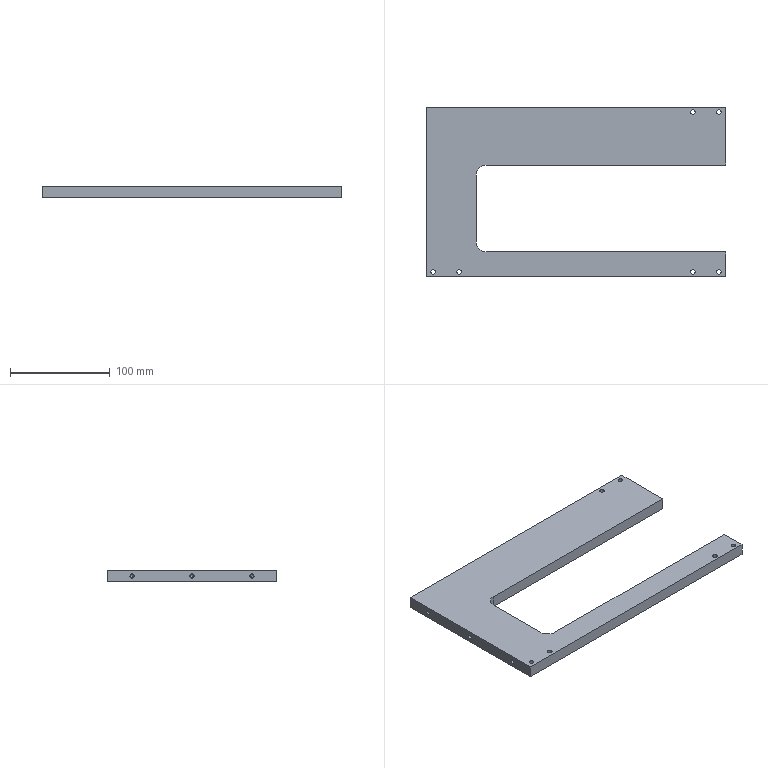Part | SolidWorks | features BaseBody 1 | 1 solid | 52 faces | box 300 x 170 x 12 mm | volume 349204 mm3 | cylinder 28 | cone 14 | plane 10 | commonest cylinder face diameters 4.134 x14 4.5 x12 20 x2